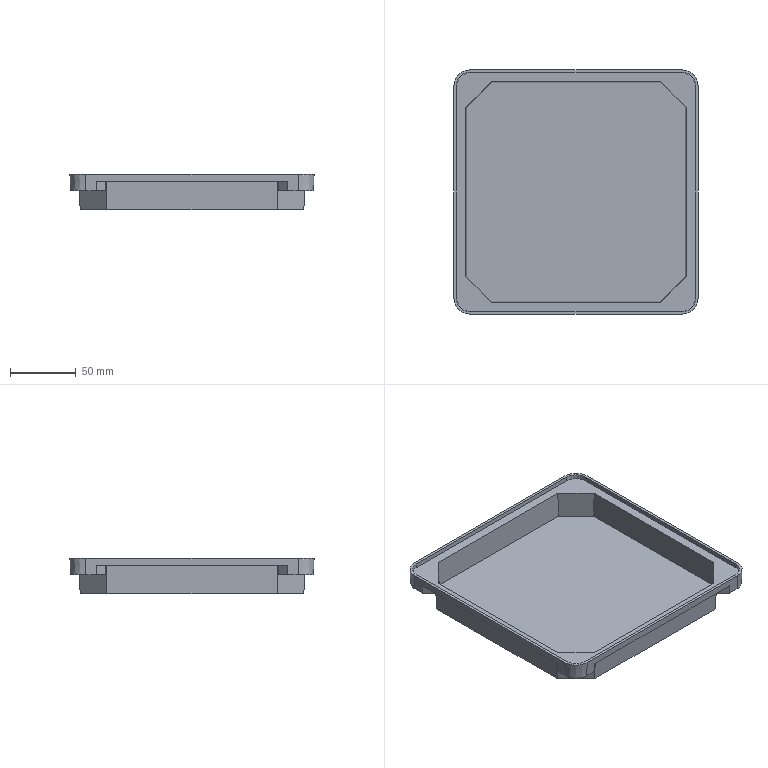Part | STEP file | Input 101 | 1 solid | 52 faces | box 186 x 186 x 27 mm | volume 135182 mm3 | plane 44 | cone 8